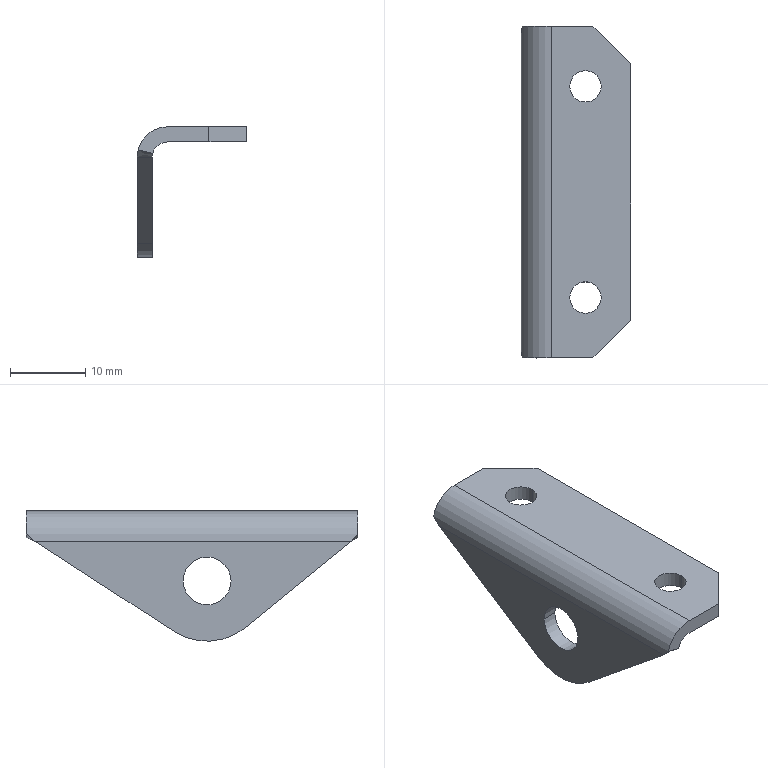Part | SolidWorks | features BaseBody 1 | 1 solid | 22 faces | box 14.5 x 44 x 17.288 mm | volume 1794 mm3 | plane 11 | cylinder 9 | spline 2 | commonest cylinder face diameters 4.17 x4 6.35 x2 4 x1 8 x1 16 x1
STEP:
#1=CARTESIAN_POINT('',(111.015,20.,2.));
#2=VERTEX_POINT('',#1);
#3=CARTESIAN_POINT('',(115.185,20.,2.));
#4=VERTEX_POINT('',#3);
#5=CARTESIAN_POINT('',(113.1,20.,2.));
#6=DIRECTION('',(0.,0.,1.));
#7=DIRECTION('',(-1.,0.,0.));
#8=AXIS2_PLACEMENT_3D('',#5,#6,#7);
#9=CIRCLE('',#8,2.085);
#10=EDGE_CURVE('',#2,#4,#9,.T.);
#11=ORIENTED_EDGE('',*,*,#10,.T.);
#12=CARTESIAN_POINT('',(115.185,20.,0.));
#13=VERTEX_POINT('',#12);
#14=CARTESIAN_POINT('',(115.185,20.,2.));
#15=DIRECTION('',(0.,0.,-1.));
#16=VECTOR('',#15,1000.);
#17=LINE('',#14,#16);
#18=EDGE_CURVE('',#4,#13,#17,.T.);
#19=ORIENTED_EDGE('',*,*,#18,.T.);
#20=CARTESIAN_POINT('',(111.015,20.,0.));
#21=VERTEX_POINT('',#20);
#22=CARTESIAN_POINT('',(113.1,20.,0.));
#23=DIRECTION('',(0.,0.,-1.));
#24=DIRECTION('',(-1.,0.,0.));
#25=AXIS2_PLACEMENT_3D('',#22,#23,#24);
#26=CIRCLE('',#25,2.085);
#27=EDGE_CURVE('',#13,#21,#26,.T.);
#28=ORIENTED_EDGE('',*,*,#27,.T.);
#29=CARTESIAN_POINT('',(111.015,20.,2.));
#30=DIRECTION('',(0.,0.,-1.));
#31=VECTOR('',#30,1000.);
#32=LINE('',#29,#31);
#33=EDGE_CURVE('',#2,#21,#32,.T.);
#34=ORIENTED_EDGE('',*,*,#33,.F.);
#35=EDGE_LOOP('',(#11,#19,#28,#34));
#36=FACE_OUTER_BOUND('',#35,.T.);
#37=CARTESIAN_POINT('',(113.1,20.,2.));
#38=DIRECTION('',(0.,0.,-1.));
#39=DIRECTION('',(-1.,0.,0.));
#40=AXIS2_PLACEMENT_3D('',#37,#38,#39);
#41=CYLINDRICAL_SURFACE('',#40,2.085);
#42=ADVANCED_FACE('',(#36),#41,.F.);
#43=CARTESIAN_POINT('',(111.015,-8.,2.));
#44=VERTEX_POINT('',#43);
#45=CARTESIAN_POINT('',(115.185,-8.,2.));
#46=VERTEX_POINT('',#45);
#47=CARTESIAN_POINT('',(113.1,-8.,2.));
#48=DIRECTION('',(0.,0.,1.));
#49=DIRECTION('',(-1.,0.,0.));
#50=AXIS2_PLACEMENT_3D('',#47,#48,#49);
#51=CIRCLE('',#50,2.085);
#52=EDGE_CURVE('',#44,#46,#51,.T.);
#53=ORIENTED_EDGE('',*,*,#52,.T.);
#54=CARTESIAN_POINT('',(115.185,-8.,0.));
#55=VERTEX_POINT('',#54);
#56=CARTESIAN_POINT('',(115.185,-8.,2.));
#57=DIRECTION('',(0.,0.,-1.));
#58=VECTOR('',#57,1000.);
#59=LINE('',#56,#58);
#60=EDGE_CURVE('',#46,#55,#59,.T.);
#61=ORIENTED_EDGE('',*,*,#60,.T.);
#62=CARTESIAN_POINT('',(111.015,-8.,0.));
#63=VERTEX_POINT('',#62);
#64=CARTESIAN_POINT('',(113.1,-8.,0.));
#65=DIRECTION('',(0.,0.,1.));
#66=DIRECTION('',(-1.,0.,0.));
#67=AXIS2_PLACEMENT_3D('',#64,#65,#66);
#68=CIRCLE('',#67,2.085);
#69=EDGE_CURVE('',#63,#55,#68,.T.);
#70=ORIENTED_EDGE('',*,*,#69,.F.);
#71=CARTESIAN_POINT('',(111.015,-8.,2.));
#72=DIRECTION('',(0.,0.,-1.));
#73=VECTOR('',#72,1000.);
#74=LINE('',#71,#73);
#75=EDGE_CURVE('',#44,#63,#74,.T.);
#76=ORIENTED_EDGE('',*,*,#75,.F.);
#77=EDGE_LOOP('',(#53,#61,#70,#76));
#78=FACE_OUTER_BOUND('',#77,.T.);
#79=CARTESIAN_POINT('',(113.1,-8.,2.));
#80=DIRECTION('',(0.,0.,-1.));
#81=DIRECTION('',(-1.,0.,0.));
#82=AXIS2_PLACEMENT_3D('',#79,#80,#81);
#83=CYLINDRICAL_SURFACE('',#82,2.085);
#84=ADVANCED_FACE('',(#78),#83,.F.);
#85=CARTESIAN_POINT('',(104.6,7.175,-7.288));
#86=VERTEX_POINT('',#85);
#87=CARTESIAN_POINT('',(104.6,0.825,-7.288));
#88=VERTEX_POINT('',#87);
#89=CARTESIAN_POINT('',(104.6,4.,-7.288));
#90=DIRECTION('',(-1.,0.,0.));
#91=DIRECTION('',(0.,1.,0.));
#92=AXIS2_PLACEMENT_3D('',#89,#90,#91);
#93=CIRCLE('',#92,3.175);
#94=EDGE_CURVE('',#86,#88,#93,.T.);
#95=ORIENTED_EDGE('',*,*,#94,.T.);
#96=CARTESIAN_POINT('',(106.6,0.825,-7.288));
#97=VERTEX_POINT('',#96);
#98=CARTESIAN_POINT('',(104.6,0.825,-7.288));
#99=DIRECTION('',(1.,0.,0.));
#100=VECTOR('',#99,1000.);
#101=LINE('',#98,#100);
#102=EDGE_CURVE('',#88,#97,#101,.T.);
#103=ORIENTED_EDGE('',*,*,#102,.T.);
#104=CARTESIAN_POINT('',(106.6,7.175,-7.288));
#105=VERTEX_POINT('',#104);
#106=CARTESIAN_POINT('',(106.6,4.,-7.288));
#107=DIRECTION('',(-1.,0.,0.));
#108=DIRECTION('',(0.,1.,0.));
#109=AXIS2_PLACEMENT_3D('',#106,#107,#108);
#110=CIRCLE('',#109,3.175);
#111=EDGE_CURVE('',#105,#97,#110,.T.);
#112=ORIENTED_EDGE('',*,*,#111,.F.);
#113=CARTESIAN_POINT('',(104.6,7.175,-7.288));
#114=DIRECTION('',(1.,0.,0.));
#115=VECTOR('',#114,1000.);
#116=LINE('',#113,#115);
#117=EDGE_CURVE('',#86,#105,#116,.T.);
#118=ORIENTED_EDGE('',*,*,#117,.F.);
#119=EDGE_LOOP('',(#95,#103,#112,#118));
#120=FACE_OUTER_BOUND('',#119,.T.);
#121=CARTESIAN_POINT('',(104.6,4.,-7.288));
#122=DIRECTION('',(1.,0.,0.));
#123=DIRECTION('',(0.,1.,0.));
#124=AXIS2_PLACEMENT_3D('',#121,#122,#123);
#125=CYLINDRICAL_SURFACE('',#124,3.175);
#126=ADVANCED_FACE('',(#120),#125,.F.);
#127=ORIENTED_EDGE('',*,*,#18,.F.);
#128=CARTESIAN_POINT('',(113.1,20.,2.));
#129=DIRECTION('',(0.,0.,1.));
#130=DIRECTION('',(-1.,0.,0.));
#131=AXIS2_PLACEMENT_3D('',#128,#129,#130);
#132=CIRCLE('',#131,2.085);
#133=EDGE_CURVE('',#4,#2,#132,.T.);
#134=ORIENTED_EDGE('',*,*,#133,.T.);
#135=ORIENTED_EDGE('',*,*,#33,.T.);
#136=CARTESIAN_POINT('',(113.1,20.,0.));
#137=DIRECTION('',(0.,0.,-1.));
#138=DIRECTION('',(-1.,0.,0.));
#139=AXIS2_PLACEMENT_3D('',#136,#137,#138);
#140=CIRCLE('',#139,2.085);
#141=EDGE_CURVE('',#21,#13,#140,.T.);
#142=ORIENTED_EDGE('',*,*,#141,.T.);
#143=EDGE_LOOP('',(#127,#134,#135,#142));
#144=FACE_OUTER_BOUND('',#143,.T.);
#145=CARTESIAN_POINT('',(113.1,20.,2.));
#146=DIRECTION('',(0.,0.,-1.));
#147=DIRECTION('',(-1.,0.,0.));
#148=AXIS2_PLACEMENT_3D('',#145,#146,#147);
#149=CYLINDRICAL_SURFACE('',#148,2.085);
#150=ADVANCED_FACE('',(#144),#149,.F.);
#151=ORIENTED_EDGE('',*,*,#141,.F.);
#152=ORIENTED_EDGE('',*,*,#27,.F.);
#153=EDGE_LOOP('',(#151,#152));
#154=FACE_BOUND('',#153,.T.);
#155=ORIENTED_EDGE('',*,*,#69,.T.);
#156=CARTESIAN_POINT('',(113.1,-8.,0.));
#157=DIRECTION('',(0.,0.,1.));
#158=DIRECTION('',(-1.,0.,0.));
#159=AXIS2_PLACEMENT_3D('',#156,#157,#158);
#160=CIRCLE('',#159,2.085);
#161=EDGE_CURVE('',#55,#63,#160,.T.);
#162=ORIENTED_EDGE('',*,*,#161,.T.);
#163=EDGE_LOOP('',(#155,#162));
#164=FACE_BOUND('',#163,.T.);
#165=CARTESIAN_POINT('',(119.1,23.,0.));
#166=VERTEX_POINT('',#165);
#167=CARTESIAN_POINT('',(119.1,-11.,0.));
#168=VERTEX_POINT('',#167);
#169=CARTESIAN_POINT('',(119.1,6.,0.));
#170=DIRECTION('',(0.,-1.,0.));
#171=VECTOR('',#170,1000.);
#172=LINE('',#169,#171);
#173=EDGE_CURVE('',#166,#168,#172,.T.);
#174=ORIENTED_EDGE('',*,*,#173,.T.);
#175=CARTESIAN_POINT('',(114.1,-16.,0.));
#176=VERTEX_POINT('',#175);
#177=CARTESIAN_POINT('',(119.1,-11.,0.));
#178=DIRECTION('',(-0.7071,-0.7071,0.));
#179=VECTOR('',#178,1000.);
#180=LINE('',#177,#179);
#181=EDGE_CURVE('',#168,#176,#180,.T.);
#182=ORIENTED_EDGE('',*,*,#181,.T.);
#183=CARTESIAN_POINT('',(108.6,-16.,0.));
#184=VERTEX_POINT('',#183);
#185=CARTESIAN_POINT('',(113.85,-16.,0.));
#186=DIRECTION('',(-1.,0.,0.));
#187=VECTOR('',#186,1000.);
#188=LINE('',#185,#187);
#189=EDGE_CURVE('',#176,#184,#188,.T.);
#190=ORIENTED_EDGE('',*,*,#189,.T.);
#191=CARTESIAN_POINT('',(108.6,28.,0.));
#192=VERTEX_POINT('',#191);
#193=CARTESIAN_POINT('',(108.6,6.,0.));
#194=DIRECTION('',(0.,1.,0.));
#195=VECTOR('',#194,1000.);
#196=LINE('',#193,#195);
#197=EDGE_CURVE('',#184,#192,#196,.T.);
#198=ORIENTED_EDGE('',*,*,#197,.T.);
#199=CARTESIAN_POINT('',(114.1,28.,0.));
#200=VERTEX_POINT('',#199);
#201=CARTESIAN_POINT('',(113.85,28.,0.));
#202=DIRECTION('',(1.,0.,0.));
#203=VECTOR('',#202,1000.);
#204=LINE('',#201,#203);
#205=EDGE_CURVE('',#192,#200,#204,.T.);
#206=ORIENTED_EDGE('',*,*,#205,.T.);
#207=CARTESIAN_POINT('',(114.1,28.,0.));
#208=DIRECTION('',(0.7071,-0.7071,0.));
#209=VECTOR('',#208,1000.);
#210=LINE('',#207,#209);
#211=EDGE_CURVE('',#200,#166,#210,.T.);
#212=ORIENTED_EDGE('',*,*,#211,.T.);
#213=EDGE_LOOP('',(#174,#182,#190,#198,#206,#212));
#214=FACE_OUTER_BOUND('',#213,.T.);
#215=CARTESIAN_POINT('',(108.6,28.,0.));
#216=DIRECTION('',(0.,0.,-1.));
#217=DIRECTION('',(1.,0.,0.));
#218=AXIS2_PLACEMENT_3D('',#215,#216,#217);
#219=PLANE('',#218);
#220=ADVANCED_FACE('',(#154,#164,#214),#219,.T.);
#221=ORIENTED_EDGE('',*,*,#52,.F.);
#222=CARTESIAN_POINT('',(113.1,-8.,2.));
#223=DIRECTION('',(0.,0.,1.));
#224=DIRECTION('',(-1.,0.,0.));
#225=AXIS2_PLACEMENT_3D('',#222,#223,#224);
#226=CIRCLE('',#225,2.085);
#227=EDGE_CURVE('',#46,#44,#226,.T.);
#228=ORIENTED_EDGE('',*,*,#227,.F.);
#229=EDGE_LOOP('',(#221,#228));
#230=FACE_BOUND('',#229,.T.);
#231=ORIENTED_EDGE('',*,*,#10,.F.);
#232=ORIENTED_EDGE('',*,*,#133,.F.);
#233=EDGE_LOOP('',(#231,#232));
#234=FACE_BOUND('',#233,.T.);
#235=CARTESIAN_POINT('',(114.1,28.,2.));
#236=VERTEX_POINT('',#235);
#237=CARTESIAN_POINT('',(119.1,23.,2.));
#238=VERTEX_POINT('',#237);
#239=CARTESIAN_POINT('',(114.1,28.,2.));
#240=DIRECTION('',(0.7071,-0.7071,0.));
#241=VECTOR('',#240,1000.);
#242=LINE('',#239,#241);
#243=EDGE_CURVE('',#236,#238,#242,.T.);
#244=ORIENTED_EDGE('',*,*,#243,.F.);
#245=CARTESIAN_POINT('',(108.6,28.,2.));
#246=VERTEX_POINT('',#245);
#247=CARTESIAN_POINT('',(113.85,28.,2.));
#248=DIRECTION('',(1.,0.,0.));
#249=VECTOR('',#248,1000.);
#250=LINE('',#247,#249);
#251=EDGE_CURVE('',#246,#236,#250,.T.);
#252=ORIENTED_EDGE('',*,*,#251,.F.);
#253=CARTESIAN_POINT('',(108.6,-16.,2.));
#254=VERTEX_POINT('',#253);
#255=CARTESIAN_POINT('',(108.6,6.,2.));
#256=DIRECTION('',(0.,1.,0.));
#257=VECTOR('',#256,1000.);
#258=LINE('',#255,#257);
#259=EDGE_CURVE('',#254,#246,#258,.T.);
#260=ORIENTED_EDGE('',*,*,#259,.F.);
#261=CARTESIAN_POINT('',(114.1,-16.,2.));
#262=VERTEX_POINT('',#261);
#263=CARTESIAN_POINT('',(113.85,-16.,2.));
#264=DIRECTION('',(-1.,0.,0.));
#265=VECTOR('',#264,1000.);
#266=LINE('',#263,#265);
#267=EDGE_CURVE('',#262,#254,#266,.T.);
#268=ORIENTED_EDGE('',*,*,#267,.F.);
#269=CARTESIAN_POINT('',(119.1,-11.,2.));
#270=VERTEX_POINT('',#269);
#271=CARTESIAN_POINT('',(119.1,-11.,2.));
#272=DIRECTION('',(-0.7071,-0.7071,0.));
#273=VECTOR('',#272,1000.);
#274=LINE('',#271,#273);
#275=EDGE_CURVE('',#270,#262,#274,.T.);
#276=ORIENTED_EDGE('',*,*,#275,.F.);
#277=CARTESIAN_POINT('',(119.1,6.,2.));
#278=DIRECTION('',(0.,-1.,0.));
#279=VECTOR('',#278,1000.);
#280=LINE('',#277,#279);
#281=EDGE_CURVE('',#238,#270,#280,.T.);
#282=ORIENTED_EDGE('',*,*,#281,.F.);
#283=EDGE_LOOP('',(#244,#252,#260,#268,#276,#282));
#284=FACE_OUTER_BOUND('',#283,.T.);
#285=CARTESIAN_POINT('',(108.6,28.,2.));
#286=DIRECTION('',(0.,0.,-1.));
#287=DIRECTION('',(1.,0.,0.));
#288=AXIS2_PLACEMENT_3D('',#285,#286,#287);
#289=PLANE('',#288);
#290=ADVANCED_FACE('',(#230,#234,#284),#289,.F.);
#291=ORIENTED_EDGE('',*,*,#60,.F.);
#292=ORIENTED_EDGE('',*,*,#227,.T.);
#293=ORIENTED_EDGE('',*,*,#75,.T.);
#294=ORIENTED_EDGE('',*,*,#161,.F.);
#295=EDGE_LOOP('',(#291,#292,#293,#294));
#296=FACE_OUTER_BOUND('',#295,.T.);
#297=CARTESIAN_POINT('',(113.1,-8.,2.));
#298=DIRECTION('',(0.,0.,-1.));
#299=DIRECTION('',(-1.,0.,0.));
#300=AXIS2_PLACEMENT_3D('',#297,#298,#299);
#301=CYLINDRICAL_SURFACE('',#300,2.085);
#302=ADVANCED_FACE('',(#296),#301,.F.);
#303=CARTESIAN_POINT('',(114.1,-16.,1.));
#304=DIRECTION('',(0.,0.,1.));
#305=VECTOR('',#304,1000.);
#306=LINE('',#303,#305);
#307=EDGE_CURVE('',#176,#262,#306,.T.);
#308=ORIENTED_EDGE('',*,*,#307,.F.);
#309=ORIENTED_EDGE('',*,*,#181,.F.);
#310=CARTESIAN_POINT('',(119.1,-11.,1.));
#311=DIRECTION('',(0.,0.,-1.));
#312=VECTOR('',#311,1000.);
#313=LINE('',#310,#312);
#314=EDGE_CURVE('',#270,#168,#313,.T.);
#315=ORIENTED_EDGE('',*,*,#314,.F.);
#316=ORIENTED_EDGE('',*,*,#275,.T.);
#317=EDGE_LOOP('',(#308,#309,#315,#316));
#318=FACE_OUTER_BOUND('',#317,.T.);
#319=CARTESIAN_POINT('',(119.1,-11.,0.));
#320=DIRECTION('',(-0.7071,0.7071,0.));
#321=DIRECTION('',(-0.7071,-0.7071,0.));
#322=AXIS2_PLACEMENT_3D('',#319,#320,#321);
#323=PLANE('',#322);
#324=ADVANCED_FACE('',(#318),#323,.F.);
#325=ORIENTED_EDGE('',*,*,#281,.T.);
#326=ORIENTED_EDGE('',*,*,#314,.T.);
#327=ORIENTED_EDGE('',*,*,#173,.F.);
#328=CARTESIAN_POINT('',(119.1,23.,1.));
#329=DIRECTION('',(0.,0.,1.));
#330=VECTOR('',#329,1000.);
#331=LINE('',#328,#330);
#332=EDGE_CURVE('',#166,#238,#331,.T.);
#333=ORIENTED_EDGE('',*,*,#332,.T.);
#334=EDGE_LOOP('',(#325,#326,#327,#333));
#335=FACE_OUTER_BOUND('',#334,.T.);
#336=CARTESIAN_POINT('',(119.1,23.,0.));
#337=DIRECTION('',(1.,0.,0.));
#338=DIRECTION('',(0.,0.,1.));
#339=AXIS2_PLACEMENT_3D('',#336,#337,#338);
#340=PLANE('',#339);
#341=ADVANCED_FACE('',(#335),#340,.T.);
#342=ORIENTED_EDGE('',*,*,#332,.F.);
#343=ORIENTED_EDGE('',*,*,#211,.F.);
#344=CARTESIAN_POINT('',(114.1,28.,1.));
#345=DIRECTION('',(0.,0.,-1.));
#346=VECTOR('',#345,1000.);
#347=LINE('',#344,#346);
#348=EDGE_CURVE('',#236,#200,#347,.T.);
#349=ORIENTED_EDGE('',*,*,#348,.F.);
#350=ORIENTED_EDGE('',*,*,#243,.T.);
#351=EDGE_LOOP('',(#342,#343,#349,#350));
#352=FACE_OUTER_BOUND('',#351,.T.);
#353=CARTESIAN_POINT('',(114.1,28.,0.));
#354=DIRECTION('',(-0.7071,-0.7071,0.));
#355=DIRECTION('',(0.7071,-0.7071,0.));
#356=AXIS2_PLACEMENT_3D('',#353,#354,#355);
#357=PLANE('',#356);
#358=ADVANCED_FACE('',(#352),#357,.F.);
#359=ORIENTED_EDGE('',*,*,#251,.T.);
#360=ORIENTED_EDGE('',*,*,#348,.T.);
#361=ORIENTED_EDGE('',*,*,#205,.F.);
#362=CARTESIAN_POINT('',(106.657,28.,-1.53));
#363=VERTEX_POINT('',#362);
#364=CARTESIAN_POINT('',(108.6,28.,-2.));
#365=DIRECTION('',(0.,1.,0.));
#366=DIRECTION('',(0.,0.,1.));
#367=AXIS2_PLACEMENT_3D('',#364,#365,#366);
#368=CIRCLE('',#367,2.);
#369=EDGE_CURVE('',#363,#192,#368,.T.);
#370=ORIENTED_EDGE('',*,*,#369,.F.);
#371=CARTESIAN_POINT('',(104.713,28.,-1.059));
#372=VERTEX_POINT('',#371);
#373=CARTESIAN_POINT('',(106.657,28.,-1.53));
#374=DIRECTION('',(-0.9719,0.,0.2352));
#375=VECTOR('',#374,1000.);
#376=LINE('',#373,#375);
#377=EDGE_CURVE('',#363,#372,#376,.T.);
#378=ORIENTED_EDGE('',*,*,#377,.T.);
#379=CARTESIAN_POINT('',(108.6,28.,-2.));
#380=DIRECTION('',(0.,1.,0.));
#381=DIRECTION('',(0.,0.,1.));
#382=AXIS2_PLACEMENT_3D('',#379,#380,#381);
#383=CIRCLE('',#382,4.);
#384=EDGE_CURVE('',#372,#246,#383,.T.);
#385=ORIENTED_EDGE('',*,*,#384,.T.);
#386=EDGE_LOOP('',(#359,#360,#361,#370,#378,#385));
#387=FACE_OUTER_BOUND('',#386,.T.);
#388=CARTESIAN_POINT('',(114.1,28.,0.));
#389=DIRECTION('',(0.,1.,0.));
#390=DIRECTION('',(-1.,0.,0.));
#391=AXIS2_PLACEMENT_3D('',#388,#389,#390);
#392=PLANE('',#391);
#393=ADVANCED_FACE('',(#387),#392,.T.);
#394=CARTESIAN_POINT('',(106.6,26.899,-2.));
#395=VERTEX_POINT('',#394);
#396=CARTESIAN_POINT('',(106.6,26.899,-2.));
#397=CARTESIAN_POINT('',(106.6,27.266,-1.842));
#398=CARTESIAN_POINT('',(106.619,27.633,-1.683));
#399=CARTESIAN_POINT('',(106.657,28.,-1.53));
#400=B_SPLINE_CURVE_WITH_KNOTS('',3,(#396,#397,#398,#399),.UNSPECIFIED.,.F.,.F.,(4,4),(0.,1.),.UNSPECIFIED.);
#401=EDGE_CURVE('',#395,#363,#400,.T.);
#402=ORIENTED_EDGE('',*,*,#401,.T.);
#403=ORIENTED_EDGE('',*,*,#369,.T.);
#404=ORIENTED_EDGE('',*,*,#197,.F.);
#405=CARTESIAN_POINT('',(106.657,-16.,-1.53));
#406=VERTEX_POINT('',#405);
#407=CARTESIAN_POINT('',(108.6,-16.,-2.));
#408=DIRECTION('',(0.,-1.,0.));
#409=DIRECTION('',(0.,0.,1.));
#410=AXIS2_PLACEMENT_3D('',#407,#408,#409);
#411=CIRCLE('',#410,2.);
#412=EDGE_CURVE('',#184,#406,#411,.T.);
#413=ORIENTED_EDGE('',*,*,#412,.T.);
#414=CARTESIAN_POINT('',(106.6,-15.127,-2.));
#415=VERTEX_POINT('',#414);
#416=CARTESIAN_POINT('',(106.657,-16.,-1.53));
#417=CARTESIAN_POINT('',(106.619,-15.709,-1.683));
#418=CARTESIAN_POINT('',(106.6,-15.418,-1.842));
#419=CARTESIAN_POINT('',(106.6,-15.127,-2.));
#420=B_SPLINE_CURVE_WITH_KNOTS('',3,(#416,#417,#418,#419),.UNSPECIFIED.,.F.,.F.,(4,4),(0.,1.),.UNSPECIFIED.);
#421=EDGE_CURVE('',#406,#415,#420,.T.);
#422=ORIENTED_EDGE('',*,*,#421,.T.);
#423=CARTESIAN_POINT('',(106.6,6.,-2.));
#424=DIRECTION('',(0.,1.,0.));
#425=VECTOR('',#424,1000.);
#426=LINE('',#423,#425);
#427=EDGE_CURVE('',#415,#395,#426,.T.);
#428=ORIENTED_EDGE('',*,*,#427,.T.);
#429=EDGE_LOOP('',(#402,#403,#404,#413,#422,#428));
#430=FACE_OUTER_BOUND('',#429,.T.);
#431=CARTESIAN_POINT('',(108.6,-16.,-2.));
#432=DIRECTION('',(0.,1.,0.));
#433=DIRECTION('',(0.,0.,1.));
#434=AXIS2_PLACEMENT_3D('',#431,#432,#433);
#435=CYLINDRICAL_SURFACE('',#434,2.);
#436=ADVANCED_FACE('',(#430),#435,.F.);
#437=ORIENTED_EDGE('',*,*,#189,.F.);
#438=ORIENTED_EDGE('',*,*,#307,.T.);
#439=ORIENTED_EDGE('',*,*,#267,.T.);
#440=CARTESIAN_POINT('',(104.713,-16.,-1.059));
#441=VERTEX_POINT('',#440);
#442=CARTESIAN_POINT('',(108.6,-16.,-2.));
#443=DIRECTION('',(0.,-1.,0.));
#444=DIRECTION('',(0.,0.,1.));
#445=AXIS2_PLACEMENT_3D('',#442,#443,#444);
#446=CIRCLE('',#445,4.);
#447=EDGE_CURVE('',#254,#441,#446,.T.);
#448=ORIENTED_EDGE('',*,*,#447,.T.);
#449=CARTESIAN_POINT('',(104.713,-16.,-1.059));
#450=DIRECTION('',(0.9719,0.,-0.2352));
#451=VECTOR('',#450,1000.);
#452=LINE('',#449,#451);
#453=EDGE_CURVE('',#441,#406,#452,.T.);
#454=ORIENTED_EDGE('',*,*,#453,.T.);
#455=ORIENTED_EDGE('',*,*,#412,.F.);
#456=EDGE_LOOP('',(#437,#438,#439,#448,#454,#455));
#457=FACE_OUTER_BOUND('',#456,.T.);
#458=CARTESIAN_POINT('',(108.6,-16.,0.));
#459=DIRECTION('',(0.,-1.,0.));
#460=DIRECTION('',(1.,0.,0.));
#461=AXIS2_PLACEMENT_3D('',#458,#459,#460);
#462=PLANE('',#461);
#463=ADVANCED_FACE('',(#457),#462,.T.);
#464=ORIENTED_EDGE('',*,*,#384,.F.);
#465=CARTESIAN_POINT('',(104.6,26.899,-2.));
#466=VERTEX_POINT('',#465);
#467=CARTESIAN_POINT('',(104.713,28.,-1.059));
#468=CARTESIAN_POINT('',(104.638,27.633,-1.367));
#469=CARTESIAN_POINT('',(104.6,27.266,-1.683));
#470=CARTESIAN_POINT('',(104.6,26.899,-2.));
#471=B_SPLINE_CURVE_WITH_KNOTS('',3,(#467,#468,#469,#470),.UNSPECIFIED.,.F.,.F.,(4,4),(0.,1.),.UNSPECIFIED.);
#472=EDGE_CURVE('',#372,#466,#471,.T.);
#473=ORIENTED_EDGE('',*,*,#472,.T.);
#474=CARTESIAN_POINT('',(104.6,-15.127,-2.));
#475=VERTEX_POINT('',#474);
#476=CARTESIAN_POINT('',(104.6,6.,-2.));
#477=DIRECTION('',(0.,1.,0.));
#478=VECTOR('',#477,1000.);
#479=LINE('',#476,#478);
#480=EDGE_CURVE('',#475,#466,#479,.T.);
#481=ORIENTED_EDGE('',*,*,#480,.F.);
#482=CARTESIAN_POINT('',(104.6,-15.127,-2.));
#483=CARTESIAN_POINT('',(104.6,-15.418,-1.683));
#484=CARTESIAN_POINT('',(104.638,-15.709,-1.367));
#485=CARTESIAN_POINT('',(104.713,-16.,-1.059));
#486=B_SPLINE_CURVE_WITH_KNOTS('',3,(#482,#483,#484,#485),.UNSPECIFIED.,.F.,.F.,(4,4),(0.,1.),.UNSPECIFIED.);
#487=EDGE_CURVE('',#475,#441,#486,.T.);
#488=ORIENTED_EDGE('',*,*,#487,.T.);
#489=ORIENTED_EDGE('',*,*,#447,.F.);
#490=ORIENTED_EDGE('',*,*,#259,.T.);
#491=EDGE_LOOP('',(#464,#473,#481,#488,#489,#490));
#492=FACE_OUTER_BOUND('',#491,.T.);
#493=CARTESIAN_POINT('',(108.6,-16.,-2.));
#494=DIRECTION('',(0.,1.,0.));
#495=DIRECTION('',(0.,0.,1.));
#496=AXIS2_PLACEMENT_3D('',#493,#494,#495);
#497=CYLINDRICAL_SURFACE('',#496,4.);
#498=ADVANCED_FACE('',(#492),#497,.T.);
#499=ORIENTED_EDGE('',*,*,#111,.T.);
#500=CARTESIAN_POINT('',(106.6,4.,-7.288));
#501=DIRECTION('',(-1.,0.,0.));
#502=DIRECTION('',(0.,1.,0.));
#503=AXIS2_PLACEMENT_3D('',#500,#501,#502);
#504=CIRCLE('',#503,3.175);
#505=EDGE_CURVE('',#97,#105,#504,.T.);
#506=ORIENTED_EDGE('',*,*,#505,.T.);
#507=EDGE_LOOP('',(#499,#506));
#508=FACE_BOUND('',#507,.T.);
#509=CARTESIAN_POINT('',(106.6,8.346,-14.004));
#510=VERTEX_POINT('',#509);
#511=CARTESIAN_POINT('',(106.6,8.346,-14.004));
#512=DIRECTION('',(0.,0.8396,0.5432));
#513=VECTOR('',#512,1000.);
#514=LINE('',#511,#513);
#515=EDGE_CURVE('',#510,#395,#514,.T.);
#516=ORIENTED_EDGE('',*,*,#515,.T.);
#517=ORIENTED_EDGE('',*,*,#427,.F.);
#518=CARTESIAN_POINT('',(106.6,-1.059,-13.485));
#519=VERTEX_POINT('',#518);
#520=CARTESIAN_POINT('',(106.6,-15.127,-2.));
#521=DIRECTION('',(0.,0.7746,-0.6324));
#522=VECTOR('',#521,1000.);
#523=LINE('',#520,#522);
#524=EDGE_CURVE('',#415,#519,#523,.T.);
#525=ORIENTED_EDGE('',*,*,#524,.T.);
#526=CARTESIAN_POINT('',(106.6,4.,-7.288));
#527=DIRECTION('',(1.,0.,0.));
#528=DIRECTION('',(0.,1.,0.));
#529=AXIS2_PLACEMENT_3D('',#526,#527,#528);
#530=CIRCLE('',#529,8.);
#531=EDGE_CURVE('',#519,#510,#530,.T.);
#532=ORIENTED_EDGE('',*,*,#531,.T.);
#533=EDGE_LOOP('',(#516,#517,#525,#532));
#534=FACE_OUTER_BOUND('',#533,.T.);
#535=CARTESIAN_POINT('',(106.6,27.151,-15.367));
#536=DIRECTION('',(1.,0.,0.));
#537=DIRECTION('',(0.,0.,1.));
#538=AXIS2_PLACEMENT_3D('',#535,#536,#537);
#539=PLANE('',#538);
#540=ADVANCED_FACE('',(#508,#534),#539,.T.);
#541=ORIENTED_EDGE('',*,*,#94,.F.);
#542=CARTESIAN_POINT('',(104.6,4.,-7.288));
#543=DIRECTION('',(-1.,0.,0.));
#544=DIRECTION('',(0.,1.,0.));
#545=AXIS2_PLACEMENT_3D('',#542,#543,#544);
#546=CIRCLE('',#545,3.175);
#547=EDGE_CURVE('',#88,#86,#546,.T.);
#548=ORIENTED_EDGE('',*,*,#547,.F.);
#549=EDGE_LOOP('',(#541,#548));
#550=FACE_BOUND('',#549,.T.);
#551=CARTESIAN_POINT('',(104.6,8.346,-14.004));
#552=VERTEX_POINT('',#551);
#553=CARTESIAN_POINT('',(104.6,26.899,-2.));
#554=DIRECTION('',(0.,0.8396,0.5432));
#555=VECTOR('',#554,1000.);
#556=LINE('',#553,#555);
#557=EDGE_CURVE('',#552,#466,#556,.T.);
#558=ORIENTED_EDGE('',*,*,#557,.F.);
#559=CARTESIAN_POINT('',(104.6,-1.059,-13.485));
#560=VERTEX_POINT('',#559);
#561=CARTESIAN_POINT('',(104.6,4.,-7.288));
#562=DIRECTION('',(1.,0.,0.));
#563=DIRECTION('',(0.,1.,0.));
#564=AXIS2_PLACEMENT_3D('',#561,#562,#563);
#565=CIRCLE('',#564,8.);
#566=EDGE_CURVE('',#560,#552,#565,.T.);
#567=ORIENTED_EDGE('',*,*,#566,.F.);
#568=CARTESIAN_POINT('',(104.6,-1.059,-13.485));
#569=DIRECTION('',(0.,0.7746,-0.6324));
#570=VECTOR('',#569,1000.);
#571=LINE('',#568,#570);
#572=EDGE_CURVE('',#475,#560,#571,.T.);
#573=ORIENTED_EDGE('',*,*,#572,.F.);
#574=ORIENTED_EDGE('',*,*,#480,.T.);
#575=EDGE_LOOP('',(#558,#567,#573,#574));
#576=FACE_OUTER_BOUND('',#575,.T.);
#577=CARTESIAN_POINT('',(104.6,27.151,-15.367));
#578=DIRECTION('',(1.,0.,0.));
#579=DIRECTION('',(0.,0.,1.));
#580=AXIS2_PLACEMENT_3D('',#577,#578,#579);
#581=PLANE('',#580);
#582=ADVANCED_FACE('',(#550,#576),#581,.F.);
#583=ORIENTED_EDGE('',*,*,#472,.F.);
#584=ORIENTED_EDGE('',*,*,#377,.F.);
#585=ORIENTED_EDGE('',*,*,#401,.F.);
#586=CARTESIAN_POINT('',(105.6,26.899,-2.));
#587=DIRECTION('',(1.,0.,0.));
#588=VECTOR('',#587,1000.);
#589=LINE('',#586,#588);
#590=EDGE_CURVE('',#466,#395,#589,.T.);
#591=ORIENTED_EDGE('',*,*,#590,.F.);
#592=EDGE_LOOP('',(#583,#584,#585,#591));
#593=FACE_OUTER_BOUND('',#592,.T.);
#594=CARTESIAN_POINT('',(104.58,26.899,-2.));
#595=CARTESIAN_POINT('',(104.58,27.266,-1.682));
#596=CARTESIAN_POINT('',(104.618,27.633,-1.364));
#597=CARTESIAN_POINT('',(104.693,28.,-1.054));
#598=CARTESIAN_POINT('',(104.6,26.899,-2.));
#599=CARTESIAN_POINT('',(104.6,27.266,-1.683));
#600=CARTESIAN_POINT('',(104.638,27.633,-1.367));
#601=CARTESIAN_POINT('',(104.713,28.,-1.059));
#602=CARTESIAN_POINT('',(106.6,26.899,-2.));
#603=CARTESIAN_POINT('',(106.6,27.266,-1.842));
#604=CARTESIAN_POINT('',(106.619,27.633,-1.683));
#605=CARTESIAN_POINT('',(106.657,28.,-1.53));
#606=B_SPLINE_SURFACE_WITH_KNOTS('',1,3,((#594,#595,#596,#597),(#598,#599,#600,#601),(#602,#603,#604,#605)),.UNSPECIFIED.,.F.,.F.,.F.,(2,1,2),(4,4),(-0.01,0.,1.),(0.,1.),.UNSPECIFIED.);
#607=ADVANCED_FACE('',(#593),#606,.F.);
#608=ORIENTED_EDGE('',*,*,#102,.F.);
#609=ORIENTED_EDGE('',*,*,#547,.T.);
#610=ORIENTED_EDGE('',*,*,#117,.T.);
#611=ORIENTED_EDGE('',*,*,#505,.F.);
#612=EDGE_LOOP('',(#608,#609,#610,#611));
#613=FACE_OUTER_BOUND('',#612,.T.);
#614=CARTESIAN_POINT('',(104.6,4.,-7.288));
#615=DIRECTION('',(1.,0.,0.));
#616=DIRECTION('',(0.,1.,0.));
#617=AXIS2_PLACEMENT_3D('',#614,#615,#616);
#618=CYLINDRICAL_SURFACE('',#617,3.175);
#619=ADVANCED_FACE('',(#613),#618,.F.);
#620=ORIENTED_EDGE('',*,*,#557,.T.);
#621=ORIENTED_EDGE('',*,*,#590,.T.);
#622=ORIENTED_EDGE('',*,*,#515,.F.);
#623=CARTESIAN_POINT('',(105.6,8.346,-14.004));
#624=DIRECTION('',(-1.,0.,0.));
#625=VECTOR('',#624,1000.);
#626=LINE('',#623,#625);
#627=EDGE_CURVE('',#510,#552,#626,.T.);
#628=ORIENTED_EDGE('',*,*,#627,.T.);
#629=EDGE_LOOP('',(#620,#621,#622,#628));
#630=FACE_OUTER_BOUND('',#629,.T.);
#631=CARTESIAN_POINT('',(106.6,26.899,-2.));
#632=DIRECTION('',(0.,0.5432,-0.8396));
#633=DIRECTION('',(0.,-0.8396,-0.5432));
#634=AXIS2_PLACEMENT_3D('',#631,#632,#633);
#635=PLANE('',#634);
#636=ADVANCED_FACE('',(#630),#635,.T.);
#637=CARTESIAN_POINT('',(105.6,-1.059,-13.485));
#638=DIRECTION('',(1.,0.,0.));
#639=VECTOR('',#638,1000.);
#640=LINE('',#637,#639);
#641=EDGE_CURVE('',#560,#519,#640,.T.);
#642=ORIENTED_EDGE('',*,*,#641,.F.);
#643=ORIENTED_EDGE('',*,*,#566,.T.);
#644=ORIENTED_EDGE('',*,*,#627,.F.);
#645=ORIENTED_EDGE('',*,*,#531,.F.);
#646=EDGE_LOOP('',(#642,#643,#644,#645));
#647=FACE_OUTER_BOUND('',#646,.T.);
#648=CARTESIAN_POINT('',(104.6,4.,-7.288));
#649=DIRECTION('',(1.,0.,0.));
#650=DIRECTION('',(0.,1.,0.));
#651=AXIS2_PLACEMENT_3D('',#648,#649,#650);
#652=CYLINDRICAL_SURFACE('',#651,8.);
#653=ADVANCED_FACE('',(#647),#652,.T.);
#654=ORIENTED_EDGE('',*,*,#524,.F.);
#655=CARTESIAN_POINT('',(105.6,-15.127,-2.));
#656=DIRECTION('',(-1.,0.,0.));
#657=VECTOR('',#656,1000.);
#658=LINE('',#655,#657);
#659=EDGE_CURVE('',#415,#475,#658,.T.);
#660=ORIENTED_EDGE('',*,*,#659,.T.);
#661=ORIENTED_EDGE('',*,*,#572,.T.);
#662=ORIENTED_EDGE('',*,*,#641,.T.);
#663=EDGE_LOOP('',(#654,#660,#661,#662));
#664=FACE_OUTER_BOUND('',#663,.T.);
#665=CARTESIAN_POINT('',(106.6,-1.059,-13.485));
#666=DIRECTION('',(0.,-0.6324,-0.7746));
#667=DIRECTION('',(0.,-0.7746,0.6324));
#668=AXIS2_PLACEMENT_3D('',#665,#666,#667);
#669=PLANE('',#668);
#670=ADVANCED_FACE('',(#664),#669,.T.);
#671=ORIENTED_EDGE('',*,*,#487,.F.);
#672=ORIENTED_EDGE('',*,*,#659,.F.);
#673=ORIENTED_EDGE('',*,*,#421,.F.);
#674=ORIENTED_EDGE('',*,*,#453,.F.);
#675=EDGE_LOOP('',(#671,#672,#673,#674));
#676=FACE_OUTER_BOUND('',#675,.T.);
#677=CARTESIAN_POINT('',(104.693,-16.,-1.054));
#678=CARTESIAN_POINT('',(104.618,-15.709,-1.364));
#679=CARTESIAN_POINT('',(104.58,-15.418,-1.682));
#680=CARTESIAN_POINT('',(104.58,-15.127,-2.));
#681=CARTESIAN_POINT('',(104.713,-16.,-1.059));
#682=CARTESIAN_POINT('',(104.638,-15.709,-1.367));
#683=CARTESIAN_POINT('',(104.6,-15.418,-1.683));
#684=CARTESIAN_POINT('',(104.6,-15.127,-2.));
#685=CARTESIAN_POINT('',(106.657,-16.,-1.53));
#686=CARTESIAN_POINT('',(106.619,-15.709,-1.683));
#687=CARTESIAN_POINT('',(106.6,-15.418,-1.842));
#688=CARTESIAN_POINT('',(106.6,-15.127,-2.));
#689=B_SPLINE_SURFACE_WITH_KNOTS('',1,3,((#677,#678,#679,#680),(#681,#682,#683,#684),(#685,#686,#687,#688)),.UNSPECIFIED.,.F.,.F.,.F.,(2,1,2),(4,4),(-0.01,0.,1.),(0.,1.),.UNSPECIFIED.);
#690=ADVANCED_FACE('',(#676),#689,.F.);
#691=CLOSED_SHELL('',(#42,#84,#126,#150,#220,#290,#302,#324,#341,#358,#393,#436,#463,#498,#540,#582,#607,#619,#636,#653,#670,#690));
#692=MANIFOLD_SOLID_BREP('',#691);
#693=CARTESIAN_POINT('',(0.,0.,0.));
#694=DIRECTION('',(0.,0.,1.));
#695=DIRECTION('',(1.,0.,0.));
#696=AXIS2_PLACEMENT_3D('',#693,#694,#695);
#697=(LENGTH_UNIT()NAMED_UNIT(*)SI_UNIT(.MILLI.,.METRE.));
#698=UNCERTAINTY_MEASURE_WITH_UNIT(LENGTH_MEASURE(0.00001),#697,'','');
#699=(NAMED_UNIT(*)PLANE_ANGLE_UNIT()SI_UNIT($,.RADIAN.));
#700=(NAMED_UNIT(*)SI_UNIT($,.STERADIAN.)SOLID_ANGLE_UNIT());
#701=(GEOMETRIC_REPRESENTATION_CONTEXT(3)GLOBAL_UNCERTAINTY_ASSIGNED_CONTEXT((#698))GLOBAL_UNIT_ASSIGNED_CONTEXT((#697,#699,#700))REPRESENTATION_CONTEXT('',''));
#702=ADVANCED_BREP_SHAPE_REPRESENTATION('',(#692,#696),#701);